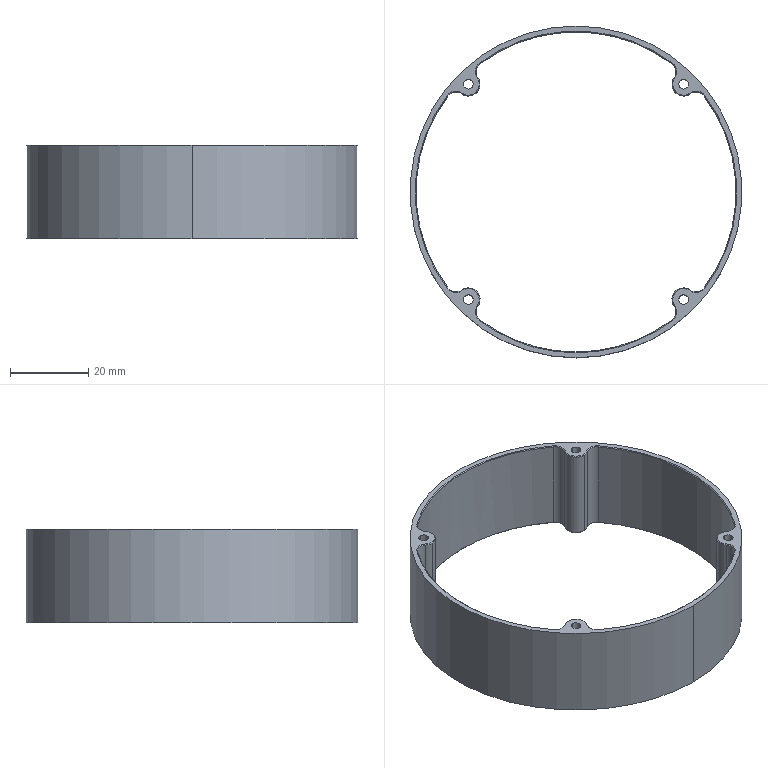Part | 1 solid | 75 faces | box 85 x 85 x 24 mm | volume 11754 mm3 | cone 42 | cylinder 31 | plane 2 | commonest cylinder face diameters 5 x10 2.5 x8 6 x6 82 x5 85 x2